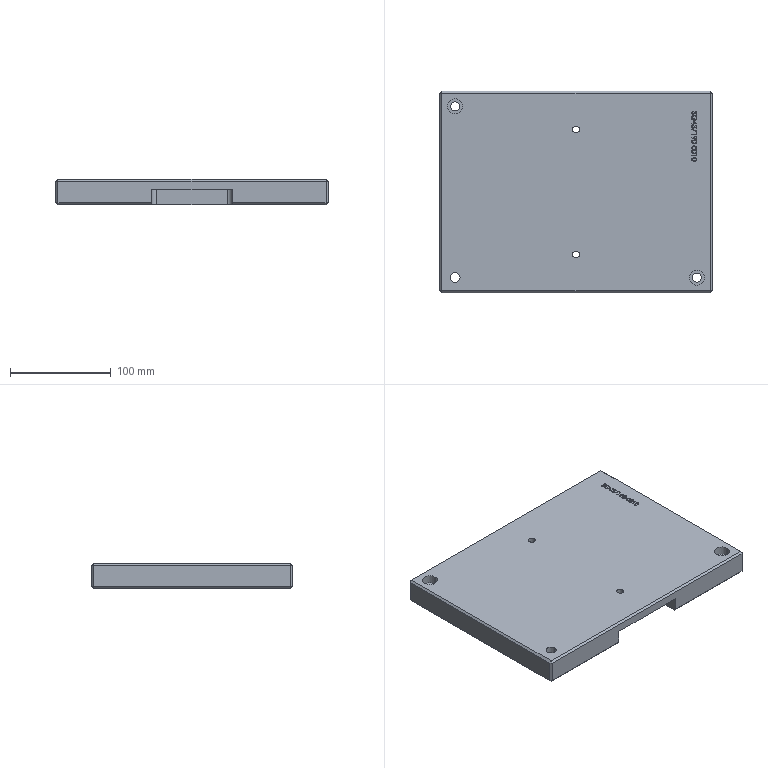Part | STEP file | Screw lock-base Mkt | 1 solid | 215 faces | box 270 x 200 x 25 mm | volume 1265515 mm3 | plane 104 | spline 83 | cylinder 18 | cone 10 | commonest cylinder face diameters 10 x6 6.8 x4 9 x4 15 x4